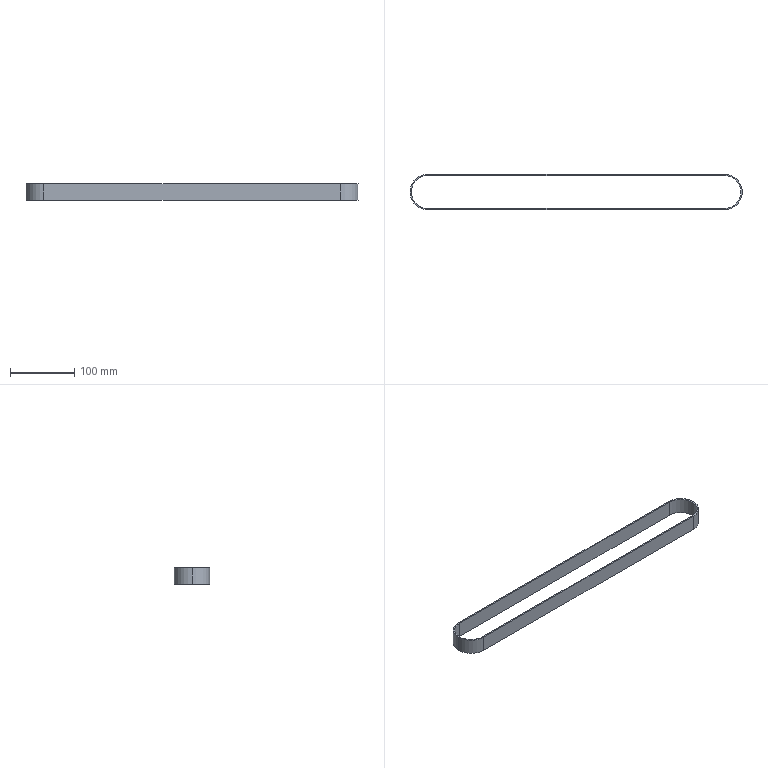Part | SolidWorks | features ExtruThin 1 | 1 solid | 12 faces | box 515 x 55 x 25 mm | volume 54325 mm3 | cylinder 6 | plane 6 | commonest cylinder face diameters 51 x3 55 x3
STEP:
#1=CARTESIAN_POINT('',(-230.,25.5,25.));
#2=VERTEX_POINT('',#1);
#3=CARTESIAN_POINT('',(-255.5,0.,25.));
#4=VERTEX_POINT('',#3);
#5=CARTESIAN_POINT('',(-230.,0.,25.));
#6=DIRECTION('',(0.,0.,1.));
#7=DIRECTION('',(1.,0.,0.));
#8=AXIS2_PLACEMENT_3D('',#5,#6,#7);
#9=CIRCLE('',#8,25.5);
#10=EDGE_CURVE('',#2,#4,#9,.T.);
#11=ORIENTED_EDGE('',*,*,#10,.T.);
#12=CARTESIAN_POINT('',(-255.5,0.,0.));
#13=VERTEX_POINT('',#12);
#14=CARTESIAN_POINT('',(-255.5,0.,25.));
#15=DIRECTION('',(0.,0.,-1.));
#16=VECTOR('',#15,1000.);
#17=LINE('',#14,#16);
#18=EDGE_CURVE('',#4,#13,#17,.T.);
#19=ORIENTED_EDGE('',*,*,#18,.T.);
#20=CARTESIAN_POINT('',(-230.,25.5,0.));
#21=VERTEX_POINT('',#20);
#22=CARTESIAN_POINT('',(-230.,0.,0.));
#23=DIRECTION('',(0.,0.,1.));
#24=DIRECTION('',(1.,0.,0.));
#25=AXIS2_PLACEMENT_3D('',#22,#23,#24);
#26=CIRCLE('',#25,25.5);
#27=EDGE_CURVE('',#21,#13,#26,.T.);
#28=ORIENTED_EDGE('',*,*,#27,.F.);
#29=CARTESIAN_POINT('',(-230.,25.5,25.));
#30=DIRECTION('',(0.,0.,-1.));
#31=VECTOR('',#30,1000.);
#32=LINE('',#29,#31);
#33=EDGE_CURVE('',#2,#21,#32,.T.);
#34=ORIENTED_EDGE('',*,*,#33,.F.);
#35=EDGE_LOOP('',(#11,#19,#28,#34));
#36=FACE_OUTER_BOUND('',#35,.T.);
#37=CARTESIAN_POINT('',(-230.,0.,25.));
#38=DIRECTION('',(0.,0.,-1.));
#39=DIRECTION('',(-1.,0.,0.));
#40=AXIS2_PLACEMENT_3D('',#37,#38,#39);
#41=CYLINDRICAL_SURFACE('',#40,25.5);
#42=ADVANCED_FACE('',(#36),#41,.F.);
#43=CARTESIAN_POINT('',(-257.5,0.,25.));
#44=VERTEX_POINT('',#43);
#45=CARTESIAN_POINT('',(-230.,-27.5,25.));
#46=VERTEX_POINT('',#45);
#47=CARTESIAN_POINT('',(-230.,0.,25.));
#48=DIRECTION('',(0.,0.,1.));
#49=DIRECTION('',(1.,0.,0.));
#50=AXIS2_PLACEMENT_3D('',#47,#48,#49);
#51=CIRCLE('',#50,27.5);
#52=EDGE_CURVE('',#44,#46,#51,.T.);
#53=ORIENTED_EDGE('',*,*,#52,.F.);
#54=CARTESIAN_POINT('',(-257.5,0.,0.));
#55=VERTEX_POINT('',#54);
#56=CARTESIAN_POINT('',(-257.5,0.,25.));
#57=DIRECTION('',(0.,0.,-1.));
#58=VECTOR('',#57,1000.);
#59=LINE('',#56,#58);
#60=EDGE_CURVE('',#44,#55,#59,.T.);
#61=ORIENTED_EDGE('',*,*,#60,.T.);
#62=CARTESIAN_POINT('',(-230.,-27.5,0.));
#63=VERTEX_POINT('',#62);
#64=CARTESIAN_POINT('',(-230.,0.,0.));
#65=DIRECTION('',(0.,0.,1.));
#66=DIRECTION('',(1.,0.,0.));
#67=AXIS2_PLACEMENT_3D('',#64,#65,#66);
#68=CIRCLE('',#67,27.5);
#69=EDGE_CURVE('',#55,#63,#68,.T.);
#70=ORIENTED_EDGE('',*,*,#69,.T.);
#71=CARTESIAN_POINT('',(-230.,-27.5,25.));
#72=DIRECTION('',(0.,0.,-1.));
#73=VECTOR('',#72,1000.);
#74=LINE('',#71,#73);
#75=EDGE_CURVE('',#46,#63,#74,.T.);
#76=ORIENTED_EDGE('',*,*,#75,.F.);
#77=EDGE_LOOP('',(#53,#61,#70,#76));
#78=FACE_OUTER_BOUND('',#77,.T.);
#79=CARTESIAN_POINT('',(-230.,0.,25.));
#80=DIRECTION('',(0.,0.,-1.));
#81=DIRECTION('',(-1.,0.,0.));
#82=AXIS2_PLACEMENT_3D('',#79,#80,#81);
#83=CYLINDRICAL_SURFACE('',#82,27.5);
#84=ADVANCED_FACE('',(#78),#83,.T.);
#85=CARTESIAN_POINT('',(-230.,27.5,25.));
#86=VERTEX_POINT('',#85);
#87=CARTESIAN_POINT('',(-230.,0.,25.));
#88=DIRECTION('',(0.,0.,1.));
#89=DIRECTION('',(1.,0.,0.));
#90=AXIS2_PLACEMENT_3D('',#87,#88,#89);
#91=CIRCLE('',#90,27.5);
#92=EDGE_CURVE('',#86,#44,#91,.T.);
#93=ORIENTED_EDGE('',*,*,#92,.T.);
#94=ORIENTED_EDGE('',*,*,#52,.T.);
#95=CARTESIAN_POINT('',(230.,-27.5,25.));
#96=VERTEX_POINT('',#95);
#97=CARTESIAN_POINT('',(-230.,-27.5,25.));
#98=DIRECTION('',(1.,0.,0.));
#99=VECTOR('',#98,1000.);
#100=LINE('',#97,#99);
#101=EDGE_CURVE('',#46,#96,#100,.T.);
#102=ORIENTED_EDGE('',*,*,#101,.T.);
#103=CARTESIAN_POINT('',(230.,27.5,25.));
#104=VERTEX_POINT('',#103);
#105=CARTESIAN_POINT('',(230.,0.,25.));
#106=DIRECTION('',(0.,0.,1.));
#107=DIRECTION('',(1.,0.,0.));
#108=AXIS2_PLACEMENT_3D('',#105,#106,#107);
#109=CIRCLE('',#108,27.5);
#110=EDGE_CURVE('',#96,#104,#109,.T.);
#111=ORIENTED_EDGE('',*,*,#110,.T.);
#112=CARTESIAN_POINT('',(-230.,27.5,25.));
#113=DIRECTION('',(-1.,0.,0.));
#114=VECTOR('',#113,1000.);
#115=LINE('',#112,#114);
#116=EDGE_CURVE('',#104,#86,#115,.T.);
#117=ORIENTED_EDGE('',*,*,#116,.T.);
#118=EDGE_LOOP('',(#93,#94,#102,#111,#117));
#119=FACE_OUTER_BOUND('',#118,.T.);
#120=CARTESIAN_POINT('',(-230.,-25.5,25.));
#121=VERTEX_POINT('',#120);
#122=CARTESIAN_POINT('',(230.,-25.5,25.));
#123=VERTEX_POINT('',#122);
#124=CARTESIAN_POINT('',(-230.,-25.5,25.));
#125=DIRECTION('',(1.,0.,0.));
#126=VECTOR('',#125,1000.);
#127=LINE('',#124,#126);
#128=EDGE_CURVE('',#121,#123,#127,.T.);
#129=ORIENTED_EDGE('',*,*,#128,.F.);
#130=CARTESIAN_POINT('',(-230.,0.,25.));
#131=DIRECTION('',(0.,0.,1.));
#132=DIRECTION('',(1.,0.,0.));
#133=AXIS2_PLACEMENT_3D('',#130,#131,#132);
#134=CIRCLE('',#133,25.5);
#135=EDGE_CURVE('',#4,#121,#134,.T.);
#136=ORIENTED_EDGE('',*,*,#135,.F.);
#137=ORIENTED_EDGE('',*,*,#10,.F.);
#138=CARTESIAN_POINT('',(230.,25.5,25.));
#139=VERTEX_POINT('',#138);
#140=CARTESIAN_POINT('',(-230.,25.5,25.));
#141=DIRECTION('',(-1.,0.,0.));
#142=VECTOR('',#141,1000.);
#143=LINE('',#140,#142);
#144=EDGE_CURVE('',#139,#2,#143,.T.);
#145=ORIENTED_EDGE('',*,*,#144,.F.);
#146=CARTESIAN_POINT('',(230.,0.,25.));
#147=DIRECTION('',(0.,0.,1.));
#148=DIRECTION('',(1.,0.,0.));
#149=AXIS2_PLACEMENT_3D('',#146,#147,#148);
#150=CIRCLE('',#149,25.5);
#151=EDGE_CURVE('',#123,#139,#150,.T.);
#152=ORIENTED_EDGE('',*,*,#151,.F.);
#153=EDGE_LOOP('',(#129,#136,#137,#145,#152));
#154=FACE_BOUND('',#153,.T.);
#155=CARTESIAN_POINT('',(-230.,0.,25.));
#156=DIRECTION('',(0.,0.,1.));
#157=DIRECTION('',(1.,0.,0.));
#158=AXIS2_PLACEMENT_3D('',#155,#156,#157);
#159=PLANE('',#158);
#160=ADVANCED_FACE('',(#119,#154),#159,.T.);
#161=CARTESIAN_POINT('',(-230.,27.5,0.));
#162=VERTEX_POINT('',#161);
#163=CARTESIAN_POINT('',(-230.,0.,0.));
#164=DIRECTION('',(0.,0.,1.));
#165=DIRECTION('',(1.,0.,0.));
#166=AXIS2_PLACEMENT_3D('',#163,#164,#165);
#167=CIRCLE('',#166,27.5);
#168=EDGE_CURVE('',#162,#55,#167,.T.);
#169=ORIENTED_EDGE('',*,*,#168,.F.);
#170=CARTESIAN_POINT('',(230.,27.5,0.));
#171=VERTEX_POINT('',#170);
#172=CARTESIAN_POINT('',(-230.,27.5,0.));
#173=DIRECTION('',(-1.,0.,0.));
#174=VECTOR('',#173,1000.);
#175=LINE('',#172,#174);
#176=EDGE_CURVE('',#171,#162,#175,.T.);
#177=ORIENTED_EDGE('',*,*,#176,.F.);
#178=CARTESIAN_POINT('',(230.,-27.5,0.));
#179=VERTEX_POINT('',#178);
#180=CARTESIAN_POINT('',(230.,0.,0.));
#181=DIRECTION('',(0.,0.,1.));
#182=DIRECTION('',(1.,0.,0.));
#183=AXIS2_PLACEMENT_3D('',#180,#181,#182);
#184=CIRCLE('',#183,27.5);
#185=EDGE_CURVE('',#179,#171,#184,.T.);
#186=ORIENTED_EDGE('',*,*,#185,.F.);
#187=CARTESIAN_POINT('',(-230.,-27.5,0.));
#188=DIRECTION('',(1.,0.,0.));
#189=VECTOR('',#188,1000.);
#190=LINE('',#187,#189);
#191=EDGE_CURVE('',#63,#179,#190,.T.);
#192=ORIENTED_EDGE('',*,*,#191,.F.);
#193=ORIENTED_EDGE('',*,*,#69,.F.);
#194=EDGE_LOOP('',(#169,#177,#186,#192,#193));
#195=FACE_OUTER_BOUND('',#194,.T.);
#196=ORIENTED_EDGE('',*,*,#27,.T.);
#197=CARTESIAN_POINT('',(-230.,-25.5,0.));
#198=VERTEX_POINT('',#197);
#199=CARTESIAN_POINT('',(-230.,0.,0.));
#200=DIRECTION('',(0.,0.,1.));
#201=DIRECTION('',(1.,0.,0.));
#202=AXIS2_PLACEMENT_3D('',#199,#200,#201);
#203=CIRCLE('',#202,25.5);
#204=EDGE_CURVE('',#13,#198,#203,.T.);
#205=ORIENTED_EDGE('',*,*,#204,.T.);
#206=CARTESIAN_POINT('',(230.,-25.5,0.));
#207=VERTEX_POINT('',#206);
#208=CARTESIAN_POINT('',(-230.,-25.5,0.));
#209=DIRECTION('',(1.,0.,0.));
#210=VECTOR('',#209,1000.);
#211=LINE('',#208,#210);
#212=EDGE_CURVE('',#198,#207,#211,.T.);
#213=ORIENTED_EDGE('',*,*,#212,.T.);
#214=CARTESIAN_POINT('',(230.,25.5,0.));
#215=VERTEX_POINT('',#214);
#216=CARTESIAN_POINT('',(230.,0.,0.));
#217=DIRECTION('',(0.,0.,1.));
#218=DIRECTION('',(1.,0.,0.));
#219=AXIS2_PLACEMENT_3D('',#216,#217,#218);
#220=CIRCLE('',#219,25.5);
#221=EDGE_CURVE('',#207,#215,#220,.T.);
#222=ORIENTED_EDGE('',*,*,#221,.T.);
#223=CARTESIAN_POINT('',(-230.,25.5,0.));
#224=DIRECTION('',(-1.,0.,0.));
#225=VECTOR('',#224,1000.);
#226=LINE('',#223,#225);
#227=EDGE_CURVE('',#215,#21,#226,.T.);
#228=ORIENTED_EDGE('',*,*,#227,.T.);
#229=EDGE_LOOP('',(#196,#205,#213,#222,#228));
#230=FACE_BOUND('',#229,.T.);
#231=CARTESIAN_POINT('',(-230.,0.,0.));
#232=DIRECTION('',(0.,0.,1.));
#233=DIRECTION('',(1.,0.,0.));
#234=AXIS2_PLACEMENT_3D('',#231,#232,#233);
#235=PLANE('',#234);
#236=ADVANCED_FACE('',(#195,#230),#235,.F.);
#237=ORIENTED_EDGE('',*,*,#60,.F.);
#238=ORIENTED_EDGE('',*,*,#92,.F.);
#239=CARTESIAN_POINT('',(-230.,27.5,25.));
#240=DIRECTION('',(0.,0.,-1.));
#241=VECTOR('',#240,1000.);
#242=LINE('',#239,#241);
#243=EDGE_CURVE('',#86,#162,#242,.T.);
#244=ORIENTED_EDGE('',*,*,#243,.T.);
#245=ORIENTED_EDGE('',*,*,#168,.T.);
#246=EDGE_LOOP('',(#237,#238,#244,#245));
#247=FACE_OUTER_BOUND('',#246,.T.);
#248=CARTESIAN_POINT('',(-230.,0.,25.));
#249=DIRECTION('',(0.,0.,-1.));
#250=DIRECTION('',(-1.,0.,0.));
#251=AXIS2_PLACEMENT_3D('',#248,#249,#250);
#252=CYLINDRICAL_SURFACE('',#251,27.5);
#253=ADVANCED_FACE('',(#247),#252,.T.);
#254=ORIENTED_EDGE('',*,*,#191,.T.);
#255=CARTESIAN_POINT('',(230.,-27.5,25.));
#256=DIRECTION('',(0.,0.,-1.));
#257=VECTOR('',#256,1000.);
#258=LINE('',#255,#257);
#259=EDGE_CURVE('',#96,#179,#258,.T.);
#260=ORIENTED_EDGE('',*,*,#259,.F.);
#261=ORIENTED_EDGE('',*,*,#101,.F.);
#262=ORIENTED_EDGE('',*,*,#75,.T.);
#263=EDGE_LOOP('',(#254,#260,#261,#262));
#264=FACE_OUTER_BOUND('',#263,.T.);
#265=CARTESIAN_POINT('',(-230.,-27.5,25.));
#266=DIRECTION('',(0.,1.,0.));
#267=DIRECTION('',(0.,0.,1.));
#268=AXIS2_PLACEMENT_3D('',#265,#266,#267);
#269=PLANE('',#268);
#270=ADVANCED_FACE('',(#264),#269,.F.);
#271=ORIENTED_EDGE('',*,*,#185,.T.);
#272=CARTESIAN_POINT('',(230.,27.5,25.));
#273=DIRECTION('',(0.,0.,-1.));
#274=VECTOR('',#273,1000.);
#275=LINE('',#272,#274);
#276=EDGE_CURVE('',#104,#171,#275,.T.);
#277=ORIENTED_EDGE('',*,*,#276,.F.);
#278=ORIENTED_EDGE('',*,*,#110,.F.);
#279=ORIENTED_EDGE('',*,*,#259,.T.);
#280=EDGE_LOOP('',(#271,#277,#278,#279));
#281=FACE_OUTER_BOUND('',#280,.T.);
#282=CARTESIAN_POINT('',(230.,0.,25.));
#283=DIRECTION('',(0.,0.,-1.));
#284=DIRECTION('',(-1.,0.,0.));
#285=AXIS2_PLACEMENT_3D('',#282,#283,#284);
#286=CYLINDRICAL_SURFACE('',#285,27.5);
#287=ADVANCED_FACE('',(#281),#286,.T.);
#288=ORIENTED_EDGE('',*,*,#176,.T.);
#289=ORIENTED_EDGE('',*,*,#243,.F.);
#290=ORIENTED_EDGE('',*,*,#116,.F.);
#291=ORIENTED_EDGE('',*,*,#276,.T.);
#292=EDGE_LOOP('',(#288,#289,#290,#291));
#293=FACE_OUTER_BOUND('',#292,.T.);
#294=CARTESIAN_POINT('',(-230.,27.5,25.));
#295=DIRECTION('',(0.,-1.,0.));
#296=DIRECTION('',(1.,0.,0.));
#297=AXIS2_PLACEMENT_3D('',#294,#295,#296);
#298=PLANE('',#297);
#299=ADVANCED_FACE('',(#293),#298,.F.);
#300=ORIENTED_EDGE('',*,*,#18,.F.);
#301=ORIENTED_EDGE('',*,*,#135,.T.);
#302=CARTESIAN_POINT('',(-230.,-25.5,25.));
#303=DIRECTION('',(0.,0.,-1.));
#304=VECTOR('',#303,1000.);
#305=LINE('',#302,#304);
#306=EDGE_CURVE('',#121,#198,#305,.T.);
#307=ORIENTED_EDGE('',*,*,#306,.T.);
#308=ORIENTED_EDGE('',*,*,#204,.F.);
#309=EDGE_LOOP('',(#300,#301,#307,#308));
#310=FACE_OUTER_BOUND('',#309,.T.);
#311=CARTESIAN_POINT('',(-230.,0.,25.));
#312=DIRECTION('',(0.,0.,-1.));
#313=DIRECTION('',(-1.,0.,0.));
#314=AXIS2_PLACEMENT_3D('',#311,#312,#313);
#315=CYLINDRICAL_SURFACE('',#314,25.5);
#316=ADVANCED_FACE('',(#310),#315,.F.);
#317=ORIENTED_EDGE('',*,*,#212,.F.);
#318=ORIENTED_EDGE('',*,*,#306,.F.);
#319=ORIENTED_EDGE('',*,*,#128,.T.);
#320=CARTESIAN_POINT('',(230.,-25.5,25.));
#321=DIRECTION('',(0.,0.,-1.));
#322=VECTOR('',#321,1000.);
#323=LINE('',#320,#322);
#324=EDGE_CURVE('',#123,#207,#323,.T.);
#325=ORIENTED_EDGE('',*,*,#324,.T.);
#326=EDGE_LOOP('',(#317,#318,#319,#325));
#327=FACE_OUTER_BOUND('',#326,.T.);
#328=CARTESIAN_POINT('',(-230.,-25.5,25.));
#329=DIRECTION('',(0.,1.,0.));
#330=DIRECTION('',(0.,0.,1.));
#331=AXIS2_PLACEMENT_3D('',#328,#329,#330);
#332=PLANE('',#331);
#333=ADVANCED_FACE('',(#327),#332,.T.);
#334=ORIENTED_EDGE('',*,*,#221,.F.);
#335=ORIENTED_EDGE('',*,*,#324,.F.);
#336=ORIENTED_EDGE('',*,*,#151,.T.);
#337=CARTESIAN_POINT('',(230.,25.5,25.));
#338=DIRECTION('',(0.,0.,-1.));
#339=VECTOR('',#338,1000.);
#340=LINE('',#337,#339);
#341=EDGE_CURVE('',#139,#215,#340,.T.);
#342=ORIENTED_EDGE('',*,*,#341,.T.);
#343=EDGE_LOOP('',(#334,#335,#336,#342));
#344=FACE_OUTER_BOUND('',#343,.T.);
#345=CARTESIAN_POINT('',(230.,0.,25.));
#346=DIRECTION('',(0.,0.,-1.));
#347=DIRECTION('',(-1.,0.,0.));
#348=AXIS2_PLACEMENT_3D('',#345,#346,#347);
#349=CYLINDRICAL_SURFACE('',#348,25.5);
#350=ADVANCED_FACE('',(#344),#349,.F.);
#351=ORIENTED_EDGE('',*,*,#227,.F.);
#352=ORIENTED_EDGE('',*,*,#341,.F.);
#353=ORIENTED_EDGE('',*,*,#144,.T.);
#354=ORIENTED_EDGE('',*,*,#33,.T.);
#355=EDGE_LOOP('',(#351,#352,#353,#354));
#356=FACE_OUTER_BOUND('',#355,.T.);
#357=CARTESIAN_POINT('',(-230.,25.5,25.));
#358=DIRECTION('',(0.,-1.,0.));
#359=DIRECTION('',(1.,0.,0.));
#360=AXIS2_PLACEMENT_3D('',#357,#358,#359);
#361=PLANE('',#360);
#362=ADVANCED_FACE('',(#356),#361,.T.);
#363=CLOSED_SHELL('',(#42,#84,#160,#236,#253,#270,#287,#299,#316,#333,#350,#362));
#364=MANIFOLD_SOLID_BREP('',#363);
#365=CARTESIAN_POINT('',(0.,0.,0.));
#366=DIRECTION('',(0.,0.,1.));
#367=DIRECTION('',(1.,0.,0.));
#368=AXIS2_PLACEMENT_3D('',#365,#366,#367);
#369=(LENGTH_UNIT()NAMED_UNIT(*)SI_UNIT(.MILLI.,.METRE.));
#370=UNCERTAINTY_MEASURE_WITH_UNIT(LENGTH_MEASURE(0.00001),#369,'','');
#371=(NAMED_UNIT(*)PLANE_ANGLE_UNIT()SI_UNIT($,.RADIAN.));
#372=(NAMED_UNIT(*)SI_UNIT($,.STERADIAN.)SOLID_ANGLE_UNIT());
#373=(GEOMETRIC_REPRESENTATION_CONTEXT(3)GLOBAL_UNCERTAINTY_ASSIGNED_CONTEXT((#370))GLOBAL_UNIT_ASSIGNED_CONTEXT((#369,#371,#372))REPRESENTATION_CONTEXT('',''));
#374=ADVANCED_BREP_SHAPE_REPRESENTATION('',(#364,#368),#373);